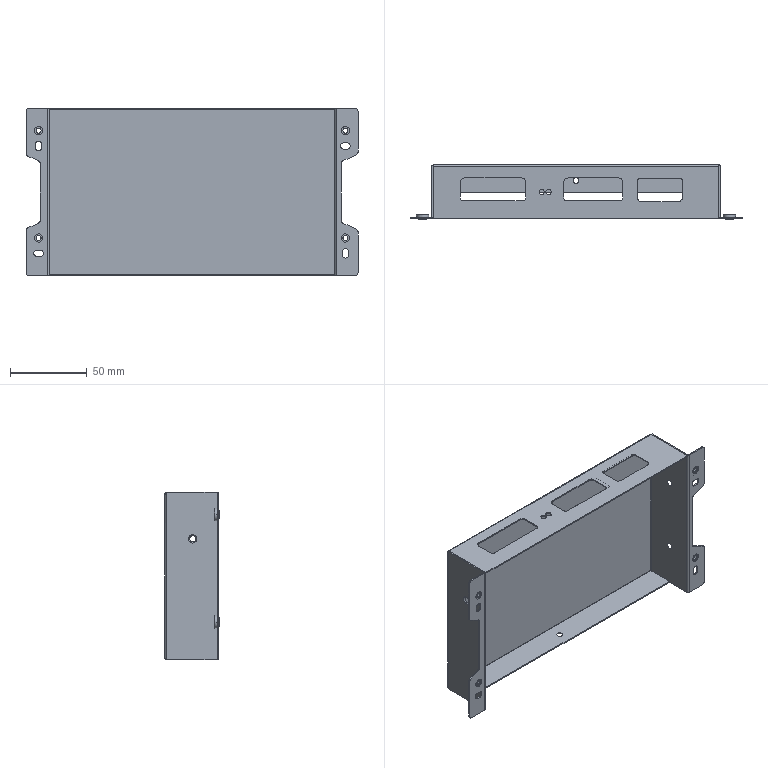Part | SolidWorks | features BaseBody 5 | 5 solids | 201 faces | box 216.4 x 35.2 x 109.5 mm | volume 30574 mm3 | cylinder 95 | plane 86 | spline 12 | cone 8 | commonest cylinder face diameters 4 x20 3.6 x11 4.2 x10 5.6 x10 3.3 x8 3.4 x8